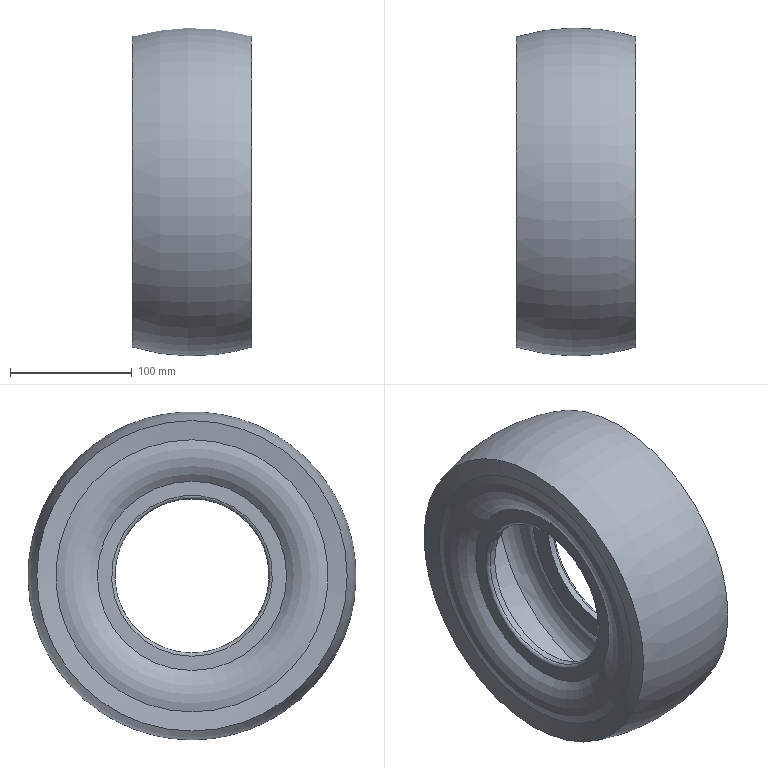Part | NX | features wheel(tire 11x4.00-5) 2 | 1 solid | 22 faces | box 97.994 x 269.588 x 269.588 mm | volume 1365848 mm3 | torus 13 | plane 4 | cone 3 | cylinder 2 | commonest cylinder face diameters 127 x2
STEP:
#1=CARTESIAN_POINT('',(48.997,0.,127.484));
#2=VERTEX_POINT('',#1);
#3=CARTESIAN_POINT('',(48.997,0.,0.));
#4=DIRECTION('',(-1.,0.,0.));
#5=DIRECTION('',(0.,0.,1.));
#6=AXIS2_PLACEMENT_3D('',#3,#4,#5);
#7=CIRCLE('',#6,127.484);
#8=EDGE_CURVE('',#2,#2,#7,.T.);
#9=ORIENTED_EDGE('',*,*,#8,.T.);
#10=EDGE_LOOP('',(#9));
#11=FACE_BOUND('',#10,.T.);
#12=CARTESIAN_POINT('',(-48.997,0.,-127.484));
#13=VERTEX_POINT('',#12);
#14=CARTESIAN_POINT('',(-48.997,0.,0.));
#15=DIRECTION('',(1.,0.,0.));
#16=DIRECTION('',(0.,0.,-1.));
#17=AXIS2_PLACEMENT_3D('',#14,#15,#16);
#18=CIRCLE('',#17,127.484);
#19=EDGE_CURVE('',#13,#13,#18,.T.);
#20=ORIENTED_EDGE('',*,*,#19,.T.);
#21=EDGE_LOOP('',(#20));
#22=FACE_BOUND('',#21,.T.);
#23=CARTESIAN_POINT('',(0.,0.,0.));
#24=DIRECTION('',(-1.,0.,0.));
#25=DIRECTION('',(0.,0.,1.));
#26=AXIS2_PLACEMENT_3D('',#23,#24,#25);
#27=DEGENERATE_TOROIDAL_SURFACE('',#26,33.063,167.857,.F.);
#28=ADVANCED_FACE('',(#11,#22),#27,.F.);
#29=CARTESIAN_POINT('',(-36.322,0.,-63.5));
#30=VERTEX_POINT('',#29);
#31=CARTESIAN_POINT('',(-36.322,0.,0.));
#32=DIRECTION('',(1.,0.,0.));
#33=DIRECTION('',(0.,0.,-1.));
#34=AXIS2_PLACEMENT_3D('',#31,#32,#33);
#35=CIRCLE('',#34,63.5);
#36=EDGE_CURVE('',#30,#30,#35,.F.);
#37=ORIENTED_EDGE('',*,*,#36,.T.);
#38=EDGE_LOOP('',(#37));
#39=FACE_BOUND('',#38,.T.);
#40=CARTESIAN_POINT('',(-30.988,0.,-63.5));
#41=VERTEX_POINT('',#40);
#42=CARTESIAN_POINT('',(-30.988,0.,0.));
#43=DIRECTION('',(1.,0.,0.));
#44=DIRECTION('',(0.,0.,-1.));
#45=AXIS2_PLACEMENT_3D('',#42,#43,#44);
#46=CIRCLE('',#45,63.5);
#47=EDGE_CURVE('',#41,#41,#46,.F.);
#48=ORIENTED_EDGE('',*,*,#47,.F.);
#49=EDGE_LOOP('',(#48));
#50=FACE_BOUND('',#49,.T.);
#51=CARTESIAN_POINT('',(0.,0.,0.));
#52=DIRECTION('',(-1.,0.,0.));
#53=DIRECTION('',(0.,0.,1.));
#54=AXIS2_PLACEMENT_3D('',#51,#52,#53);
#55=CYLINDRICAL_SURFACE('',#54,63.5);
#56=ADVANCED_FACE('',(#39,#50),#55,.F.);
#57=CARTESIAN_POINT('',(46.914,0.,111.76));
#58=VERTEX_POINT('',#57);
#59=CARTESIAN_POINT('',(46.914,0.,0.));
#60=DIRECTION('',(-1.,0.,0.));
#61=DIRECTION('',(0.,0.,1.));
#62=AXIS2_PLACEMENT_3D('',#59,#60,#61);
#63=CIRCLE('',#62,111.76);
#64=EDGE_CURVE('',#58,#58,#63,.T.);
#65=ORIENTED_EDGE('',*,*,#64,.T.);
#66=EDGE_LOOP('',(#65));
#67=FACE_BOUND('',#66,.T.);
#68=ORIENTED_EDGE('',*,*,#8,.F.);
#69=EDGE_LOOP('',(#68));
#70=FACE_BOUND('',#69,.T.);
#71=CARTESIAN_POINT('',(46.914,0.,0.));
#72=DIRECTION('',(1.,0.,0.));
#73=DIRECTION('',(0.,0.,-1.));
#74=AXIS2_PLACEMENT_3D('',#71,#72,#73);
#75=CONICAL_SURFACE('',#74,111.76,1.439);
#76=ADVANCED_FACE('',(#67,#70),#75,.F.);
#77=ORIENTED_EDGE('',*,*,#64,.F.);
#78=EDGE_LOOP('',(#77));
#79=FACE_BOUND('',#78,.T.);
#80=CARTESIAN_POINT('',(38.862,0.,77.724));
#81=VERTEX_POINT('',#80);
#82=CARTESIAN_POINT('',(38.862,0.,0.));
#83=DIRECTION('',(-1.,0.,0.));
#84=DIRECTION('',(0.,0.,1.));
#85=AXIS2_PLACEMENT_3D('',#82,#83,#84);
#86=CIRCLE('',#85,77.724);
#87=EDGE_CURVE('',#81,#81,#86,.T.);
#88=ORIENTED_EDGE('',*,*,#87,.T.);
#89=EDGE_LOOP('',(#88));
#90=FACE_BOUND('',#89,.T.);
#91=CARTESIAN_POINT('',(15.83,0.,0.));
#92=DIRECTION('',(-1.,0.,0.));
#93=DIRECTION('',(0.,0.,1.));
#94=AXIS2_PLACEMENT_3D('',#91,#92,#93);
#95=TOROIDAL_SURFACE('',#94,101.143,32.847);
#96=ADVANCED_FACE('',(#79,#90),#95,.T.);
#97=CARTESIAN_POINT('',(38.862,0.,66.04));
#98=VERTEX_POINT('',#97);
#99=CARTESIAN_POINT('',(38.862,0.,0.));
#100=DIRECTION('',(-1.,0.,0.));
#101=DIRECTION('',(0.,0.,1.));
#102=AXIS2_PLACEMENT_3D('',#99,#100,#101);
#103=CIRCLE('',#102,66.04);
#104=EDGE_CURVE('',#98,#98,#103,.T.);
#105=ORIENTED_EDGE('',*,*,#104,.T.);
#106=EDGE_LOOP('',(#105));
#107=FACE_BOUND('',#106,.T.);
#108=ORIENTED_EDGE('',*,*,#87,.F.);
#109=EDGE_LOOP('',(#108));
#110=FACE_BOUND('',#109,.T.);
#111=CARTESIAN_POINT('',(38.862,63.5,0.));
#112=DIRECTION('',(-1.,0.,0.));
#113=DIRECTION('',(0.,0.,1.));
#114=AXIS2_PLACEMENT_3D('',#111,#112,#113);
#115=PLANE('',#114);
#116=ADVANCED_FACE('',(#107,#110),#115,.F.);
#117=CARTESIAN_POINT('',(36.322,0.,63.5));
#118=VERTEX_POINT('',#117);
#119=CARTESIAN_POINT('',(36.322,0.,0.));
#120=DIRECTION('',(-1.,0.,0.));
#121=DIRECTION('',(0.,0.,1.));
#122=AXIS2_PLACEMENT_3D('',#119,#120,#121);
#123=CIRCLE('',#122,63.5);
#124=EDGE_CURVE('',#118,#118,#123,.F.);
#125=ORIENTED_EDGE('',*,*,#124,.T.);
#126=EDGE_LOOP('',(#125));
#127=FACE_BOUND('',#126,.T.);
#128=CARTESIAN_POINT('',(30.988,0.,63.5));
#129=VERTEX_POINT('',#128);
#130=CARTESIAN_POINT('',(30.988,0.,0.));
#131=DIRECTION('',(-1.,0.,0.));
#132=DIRECTION('',(0.,0.,1.));
#133=AXIS2_PLACEMENT_3D('',#130,#131,#132);
#134=CIRCLE('',#133,63.5);
#135=EDGE_CURVE('',#129,#129,#134,.T.);
#136=ORIENTED_EDGE('',*,*,#135,.T.);
#137=EDGE_LOOP('',(#136));
#138=FACE_BOUND('',#137,.T.);
#139=CARTESIAN_POINT('',(0.,0.,0.));
#140=DIRECTION('',(-1.,0.,0.));
#141=DIRECTION('',(0.,0.,1.));
#142=AXIS2_PLACEMENT_3D('',#139,#140,#141);
#143=CYLINDRICAL_SURFACE('',#142,63.5);
#144=ADVANCED_FACE('',(#127,#138),#143,.F.);
#145=CARTESIAN_POINT('',(-46.914,0.,111.76));
#146=VERTEX_POINT('',#145);
#147=CARTESIAN_POINT('',(-46.914,0.,0.));
#148=DIRECTION('',(-1.,0.,0.));
#149=DIRECTION('',(0.,0.,1.));
#150=AXIS2_PLACEMENT_3D('',#147,#148,#149);
#151=CIRCLE('',#150,111.76);
#152=EDGE_CURVE('',#146,#146,#151,.T.);
#153=ORIENTED_EDGE('',*,*,#152,.F.);
#154=EDGE_LOOP('',(#153));
#155=FACE_BOUND('',#154,.T.);
#156=ORIENTED_EDGE('',*,*,#19,.F.);
#157=EDGE_LOOP('',(#156));
#158=FACE_BOUND('',#157,.T.);
#159=CARTESIAN_POINT('',(-46.914,0.,0.));
#160=DIRECTION('',(-1.,0.,0.));
#161=DIRECTION('',(0.,0.,-1.));
#162=AXIS2_PLACEMENT_3D('',#159,#160,#161);
#163=CONICAL_SURFACE('',#162,111.76,1.439);
#164=ADVANCED_FACE('',(#155,#158),#163,.F.);
#165=ORIENTED_EDGE('',*,*,#152,.T.);
#166=EDGE_LOOP('',(#165));
#167=FACE_BOUND('',#166,.T.);
#168=CARTESIAN_POINT('',(-38.862,0.,77.724));
#169=VERTEX_POINT('',#168);
#170=CARTESIAN_POINT('',(-38.862,0.,0.));
#171=DIRECTION('',(-1.,0.,0.));
#172=DIRECTION('',(0.,0.,1.));
#173=AXIS2_PLACEMENT_3D('',#170,#171,#172);
#174=CIRCLE('',#173,77.724);
#175=EDGE_CURVE('',#169,#169,#174,.T.);
#176=ORIENTED_EDGE('',*,*,#175,.F.);
#177=EDGE_LOOP('',(#176));
#178=FACE_BOUND('',#177,.T.);
#179=CARTESIAN_POINT('',(-15.83,0.,0.));
#180=DIRECTION('',(1.,0.,0.));
#181=DIRECTION('',(0.,0.,1.));
#182=AXIS2_PLACEMENT_3D('',#179,#180,#181);
#183=TOROIDAL_SURFACE('',#182,101.143,32.847);
#184=ADVANCED_FACE('',(#167,#178),#183,.T.);
#185=CARTESIAN_POINT('',(-38.862,0.,-66.04));
#186=VERTEX_POINT('',#185);
#187=CARTESIAN_POINT('',(-38.862,0.,0.));
#188=DIRECTION('',(1.,0.,0.));
#189=DIRECTION('',(0.,0.,-1.));
#190=AXIS2_PLACEMENT_3D('',#187,#188,#189);
#191=CIRCLE('',#190,66.04);
#192=EDGE_CURVE('',#186,#186,#191,.T.);
#193=ORIENTED_EDGE('',*,*,#192,.T.);
#194=EDGE_LOOP('',(#193));
#195=FACE_BOUND('',#194,.T.);
#196=ORIENTED_EDGE('',*,*,#175,.T.);
#197=EDGE_LOOP('',(#196));
#198=FACE_BOUND('',#197,.T.);
#199=CARTESIAN_POINT('',(-38.862,63.5,0.));
#200=DIRECTION('',(1.,0.,0.));
#201=DIRECTION('',(0.,0.,1.));
#202=AXIS2_PLACEMENT_3D('',#199,#200,#201);
#203=PLANE('',#202);
#204=ADVANCED_FACE('',(#195,#198),#203,.F.);
#205=CARTESIAN_POINT('',(30.257,0.,121.527));
#206=VERTEX_POINT('',#205);
#207=CARTESIAN_POINT('',(30.257,0.,0.));
#208=DIRECTION('',(-1.,0.,0.));
#209=DIRECTION('',(0.,0.,1.));
#210=AXIS2_PLACEMENT_3D('',#207,#208,#209);
#211=CIRCLE('',#210,121.527);
#212=EDGE_CURVE('',#206,#206,#211,.T.);
#213=ORIENTED_EDGE('',*,*,#212,.F.);
#214=EDGE_LOOP('',(#213));
#215=FACE_BOUND('',#214,.T.);
#216=CARTESIAN_POINT('',(-33.847,0.,-120.781));
#217=VERTEX_POINT('',#216);
#218=CARTESIAN_POINT('',(-33.847,0.,0.));
#219=DIRECTION('',(1.,0.,0.));
#220=DIRECTION('',(0.,0.,-1.));
#221=AXIS2_PLACEMENT_3D('',#218,#219,#220);
#222=CIRCLE('',#221,120.781);
#223=EDGE_CURVE('',#217,#217,#222,.F.);
#224=ORIENTED_EDGE('',*,*,#223,.T.);
#225=EDGE_LOOP('',(#224));
#226=FACE_BOUND('',#225,.T.);
#227=CARTESIAN_POINT('',(0.,0.,0.));
#228=DIRECTION('',(-1.,0.,0.));
#229=DIRECTION('',(0.,0.,1.));
#230=AXIS2_PLACEMENT_3D('',#227,#228,#229);
#231=DEGENERATE_TOROIDAL_SURFACE('',#230,33.063,157.523,.F.);
#232=ADVANCED_FACE('',(#215,#226),#231,.T.);
#233=CARTESIAN_POINT('',(31.894,0.,82.023));
#234=VERTEX_POINT('',#233);
#235=CARTESIAN_POINT('',(31.894,0.,0.));
#236=DIRECTION('',(-1.,0.,0.));
#237=DIRECTION('',(0.,0.,1.));
#238=AXIS2_PLACEMENT_3D('',#235,#236,#237);
#239=CIRCLE('',#238,82.023);
#240=EDGE_CURVE('',#234,#234,#239,.F.);
#241=ORIENTED_EDGE('',*,*,#240,.T.);
#242=EDGE_LOOP('',(#241));
#243=FACE_BOUND('',#242,.T.);
#244=ORIENTED_EDGE('',*,*,#212,.T.);
#245=EDGE_LOOP('',(#244));
#246=FACE_BOUND('',#245,.T.);
#247=CARTESIAN_POINT('',(15.83,0.,0.));
#248=DIRECTION('',(-1.,0.,0.));
#249=DIRECTION('',(0.,0.,1.));
#250=AXIS2_PLACEMENT_3D('',#247,#248,#249);
#251=TOROIDAL_SURFACE('',#250,101.143,24.973);
#252=ADVANCED_FACE('',(#243,#246),#251,.F.);
#253=CARTESIAN_POINT('',(30.988,0.,80.078));
#254=VERTEX_POINT('',#253);
#255=CARTESIAN_POINT('',(30.988,0.,0.));
#256=DIRECTION('',(-1.,0.,0.));
#257=DIRECTION('',(0.,0.,1.));
#258=AXIS2_PLACEMENT_3D('',#255,#256,#257);
#259=CIRCLE('',#258,80.078);
#260=EDGE_CURVE('',#254,#254,#259,.T.);
#261=ORIENTED_EDGE('',*,*,#260,.T.);
#262=EDGE_LOOP('',(#261));
#263=FACE_BOUND('',#262,.T.);
#264=ORIENTED_EDGE('',*,*,#135,.F.);
#265=EDGE_LOOP('',(#264));
#266=FACE_BOUND('',#265,.T.);
#267=CARTESIAN_POINT('',(30.988,63.5,0.));
#268=DIRECTION('',(-1.,0.,0.));
#269=DIRECTION('',(0.,0.,1.));
#270=AXIS2_PLACEMENT_3D('',#267,#268,#269);
#271=PLANE('',#270);
#272=ADVANCED_FACE('',(#263,#266),#271,.T.);
#273=CARTESIAN_POINT('',(-36.074,0.,-119.967));
#274=VERTEX_POINT('',#273);
#275=CARTESIAN_POINT('',(-36.074,0.,0.));
#276=DIRECTION('',(1.,0.,0.));
#277=DIRECTION('',(0.,0.,-1.));
#278=AXIS2_PLACEMENT_3D('',#275,#276,#277);
#279=CIRCLE('',#278,119.967);
#280=EDGE_CURVE('',#274,#274,#279,.F.);
#281=ORIENTED_EDGE('',*,*,#280,.T.);
#282=EDGE_LOOP('',(#281));
#283=FACE_BOUND('',#282,.T.);
#284=ORIENTED_EDGE('',*,*,#223,.F.);
#285=EDGE_LOOP('',(#284));
#286=FACE_BOUND('',#285,.T.);
#287=CARTESIAN_POINT('',(-31.937,0.,0.));
#288=DIRECTION('',(1.,0.,0.));
#289=DIRECTION('',(0.,0.,1.));
#290=AXIS2_PLACEMENT_3D('',#287,#288,#289);
#291=TOROIDAL_SURFACE('',#290,112.098,8.89);
#292=ADVANCED_FACE('',(#283,#286),#291,.F.);
#293=CARTESIAN_POINT('',(-37.128,0.,-115.252));
#294=VERTEX_POINT('',#293);
#295=CARTESIAN_POINT('',(-37.128,0.,0.));
#296=DIRECTION('',(1.,0.,0.));
#297=DIRECTION('',(0.,0.,-1.));
#298=AXIS2_PLACEMENT_3D('',#295,#296,#297);
#299=CIRCLE('',#298,115.252);
#300=EDGE_CURVE('',#294,#294,#299,.F.);
#301=ORIENTED_EDGE('',*,*,#300,.T.);
#302=EDGE_LOOP('',(#301));
#303=FACE_BOUND('',#302,.T.);
#304=CARTESIAN_POINT('',(-37.41,0.,117.385));
#305=VERTEX_POINT('',#304);
#306=CARTESIAN_POINT('',(-37.41,0.,0.));
#307=DIRECTION('',(-1.,0.,0.));
#308=DIRECTION('',(0.,0.,1.));
#309=AXIS2_PLACEMENT_3D('',#306,#307,#308);
#310=CIRCLE('',#309,117.385);
#311=EDGE_CURVE('',#305,#305,#310,.F.);
#312=ORIENTED_EDGE('',*,*,#311,.T.);
#313=EDGE_LOOP('',(#312));
#314=FACE_BOUND('',#313,.T.);
#315=CARTESIAN_POINT('',(-36.842,0.,0.));
#316=DIRECTION('',(-1.,0.,0.));
#317=DIRECTION('',(0.,0.,-1.));
#318=AXIS2_PLACEMENT_3D('',#315,#316,#317);
#319=CONICAL_SURFACE('',#318,113.095,1.439);
#320=ADVANCED_FACE('',(#303,#314),#319,.T.);
#321=CARTESIAN_POINT('',(-31.894,0.,-82.023));
#322=VERTEX_POINT('',#321);
#323=CARTESIAN_POINT('',(-31.894,0.,0.));
#324=DIRECTION('',(1.,0.,0.));
#325=DIRECTION('',(0.,0.,-1.));
#326=AXIS2_PLACEMENT_3D('',#323,#324,#325);
#327=CIRCLE('',#326,82.023);
#328=EDGE_CURVE('',#322,#322,#327,.F.);
#329=ORIENTED_EDGE('',*,*,#328,.T.);
#330=EDGE_LOOP('',(#329));
#331=FACE_BOUND('',#330,.T.);
#332=CARTESIAN_POINT('',(-37.447,0.,-113.647));
#333=VERTEX_POINT('',#332);
#334=CARTESIAN_POINT('',(-37.447,0.,0.));
#335=DIRECTION('',(1.,0.,0.));
#336=DIRECTION('',(0.,0.,-1.));
#337=AXIS2_PLACEMENT_3D('',#334,#335,#336);
#338=CIRCLE('',#337,113.647);
#339=EDGE_CURVE('',#333,#333,#338,.T.);
#340=ORIENTED_EDGE('',*,*,#339,.T.);
#341=EDGE_LOOP('',(#340));
#342=FACE_BOUND('',#341,.T.);
#343=CARTESIAN_POINT('',(-15.83,0.,0.));
#344=DIRECTION('',(1.,0.,0.));
#345=DIRECTION('',(0.,0.,1.));
#346=AXIS2_PLACEMENT_3D('',#343,#344,#345);
#347=TOROIDAL_SURFACE('',#346,101.143,24.973);
#348=ADVANCED_FACE('',(#331,#342),#347,.F.);
#349=CARTESIAN_POINT('',(-30.988,0.,-80.078));
#350=VERTEX_POINT('',#349);
#351=CARTESIAN_POINT('',(-30.988,0.,0.));
#352=DIRECTION('',(1.,0.,0.));
#353=DIRECTION('',(0.,0.,-1.));
#354=AXIS2_PLACEMENT_3D('',#351,#352,#353);
#355=CIRCLE('',#354,80.078);
#356=EDGE_CURVE('',#350,#350,#355,.T.);
#357=ORIENTED_EDGE('',*,*,#356,.T.);
#358=EDGE_LOOP('',(#357));
#359=FACE_BOUND('',#358,.T.);
#360=ORIENTED_EDGE('',*,*,#47,.T.);
#361=EDGE_LOOP('',(#360));
#362=FACE_BOUND('',#361,.T.);
#363=CARTESIAN_POINT('',(-30.988,63.5,0.));
#364=DIRECTION('',(1.,0.,0.));
#365=DIRECTION('',(0.,0.,1.));
#366=AXIS2_PLACEMENT_3D('',#363,#364,#365);
#367=PLANE('',#366);
#368=ADVANCED_FACE('',(#359,#362),#367,.T.);
#369=ORIENTED_EDGE('',*,*,#124,.F.);
#370=EDGE_LOOP('',(#369));
#371=FACE_BOUND('',#370,.T.);
#372=ORIENTED_EDGE('',*,*,#104,.F.);
#373=EDGE_LOOP('',(#372));
#374=FACE_BOUND('',#373,.T.);
#375=CARTESIAN_POINT('',(36.322,0.,0.));
#376=DIRECTION('',(-1.,0.,0.));
#377=DIRECTION('',(0.,0.,1.));
#378=AXIS2_PLACEMENT_3D('',#375,#376,#377);
#379=TOROIDAL_SURFACE('',#378,66.04,2.54);
#380=ADVANCED_FACE('',(#371,#374),#379,.T.);
#381=ORIENTED_EDGE('',*,*,#192,.F.);
#382=EDGE_LOOP('',(#381));
#383=FACE_BOUND('',#382,.T.);
#384=ORIENTED_EDGE('',*,*,#36,.F.);
#385=EDGE_LOOP('',(#384));
#386=FACE_BOUND('',#385,.T.);
#387=CARTESIAN_POINT('',(-36.322,0.,0.));
#388=DIRECTION('',(1.,0.,0.));
#389=DIRECTION('',(0.,0.,-1.));
#390=AXIS2_PLACEMENT_3D('',#387,#388,#389);
#391=TOROIDAL_SURFACE('',#390,66.04,2.54);
#392=ADVANCED_FACE('',(#383,#386),#391,.T.);
#393=ORIENTED_EDGE('',*,*,#356,.F.);
#394=EDGE_LOOP('',(#393));
#395=FACE_BOUND('',#394,.T.);
#396=ORIENTED_EDGE('',*,*,#328,.F.);
#397=EDGE_LOOP('',(#396));
#398=FACE_BOUND('',#397,.T.);
#399=CARTESIAN_POINT('',(-33.528,0.,0.));
#400=DIRECTION('',(-1.,0.,0.));
#401=DIRECTION('',(0.,0.,1.));
#402=AXIS2_PLACEMENT_3D('',#399,#400,#401);
#403=TOROIDAL_SURFACE('',#402,80.078,2.54);
#404=ADVANCED_FACE('',(#395,#398),#403,.T.);
#405=ORIENTED_EDGE('',*,*,#339,.F.);
#406=EDGE_LOOP('',(#405));
#407=FACE_BOUND('',#406,.T.);
#408=ORIENTED_EDGE('',*,*,#300,.F.);
#409=EDGE_LOOP('',(#408));
#410=FACE_BOUND('',#409,.T.);
#411=CARTESIAN_POINT('',(-39.646,0.,0.));
#412=DIRECTION('',(1.,0.,0.));
#413=DIRECTION('',(0.,0.,-1.));
#414=AXIS2_PLACEMENT_3D('',#411,#412,#413);
#415=TOROIDAL_SURFACE('',#414,114.919,2.54);
#416=ADVANCED_FACE('',(#407,#410),#415,.T.);
#417=ORIENTED_EDGE('',*,*,#311,.F.);
#418=EDGE_LOOP('',(#417));
#419=FACE_BOUND('',#418,.T.);
#420=ORIENTED_EDGE('',*,*,#280,.F.);
#421=EDGE_LOOP('',(#420));
#422=FACE_BOUND('',#421,.T.);
#423=CARTESIAN_POINT('',(-34.892,0.,0.));
#424=DIRECTION('',(-1.,0.,0.));
#425=DIRECTION('',(0.,0.,1.));
#426=AXIS2_PLACEMENT_3D('',#423,#424,#425);
#427=TOROIDAL_SURFACE('',#426,117.719,2.54);
#428=ADVANCED_FACE('',(#419,#422),#427,.F.);
#429=ORIENTED_EDGE('',*,*,#240,.F.);
#430=EDGE_LOOP('',(#429));
#431=FACE_BOUND('',#430,.T.);
#432=ORIENTED_EDGE('',*,*,#260,.F.);
#433=EDGE_LOOP('',(#432));
#434=FACE_BOUND('',#433,.T.);
#435=CARTESIAN_POINT('',(33.528,0.,0.));
#436=DIRECTION('',(1.,0.,0.));
#437=DIRECTION('',(0.,0.,-1.));
#438=AXIS2_PLACEMENT_3D('',#435,#436,#437);
#439=TOROIDAL_SURFACE('',#438,80.078,2.54);
#440=ADVANCED_FACE('',(#431,#434),#439,.T.);
#441=CLOSED_SHELL('',(#28,#56,#76,#96,#116,#144,#164,#184,#204,#232,#252,#272,#292,#320,#348,#368,#380,#392,#404,#416,#428,#440));
#442=MANIFOLD_SOLID_BREP('',#441);
#443=(LENGTH_UNIT()NAMED_UNIT(*)SI_UNIT(.MILLI.,.METRE.));
#444=UNCERTAINTY_MEASURE_WITH_UNIT(LENGTH_MEASURE(0.00001),#443,'','');
#445=(NAMED_UNIT(*)PLANE_ANGLE_UNIT()SI_UNIT($,.RADIAN.));
#446=(NAMED_UNIT(*)SI_UNIT($,.STERADIAN.)SOLID_ANGLE_UNIT());
#447=(GEOMETRIC_REPRESENTATION_CONTEXT(3)GLOBAL_UNCERTAINTY_ASSIGNED_CONTEXT((#444))GLOBAL_UNIT_ASSIGNED_CONTEXT((#443,#445,#446))REPRESENTATION_CONTEXT('',''));
#448=ADVANCED_BREP_SHAPE_REPRESENTATION('',(#442),#447);